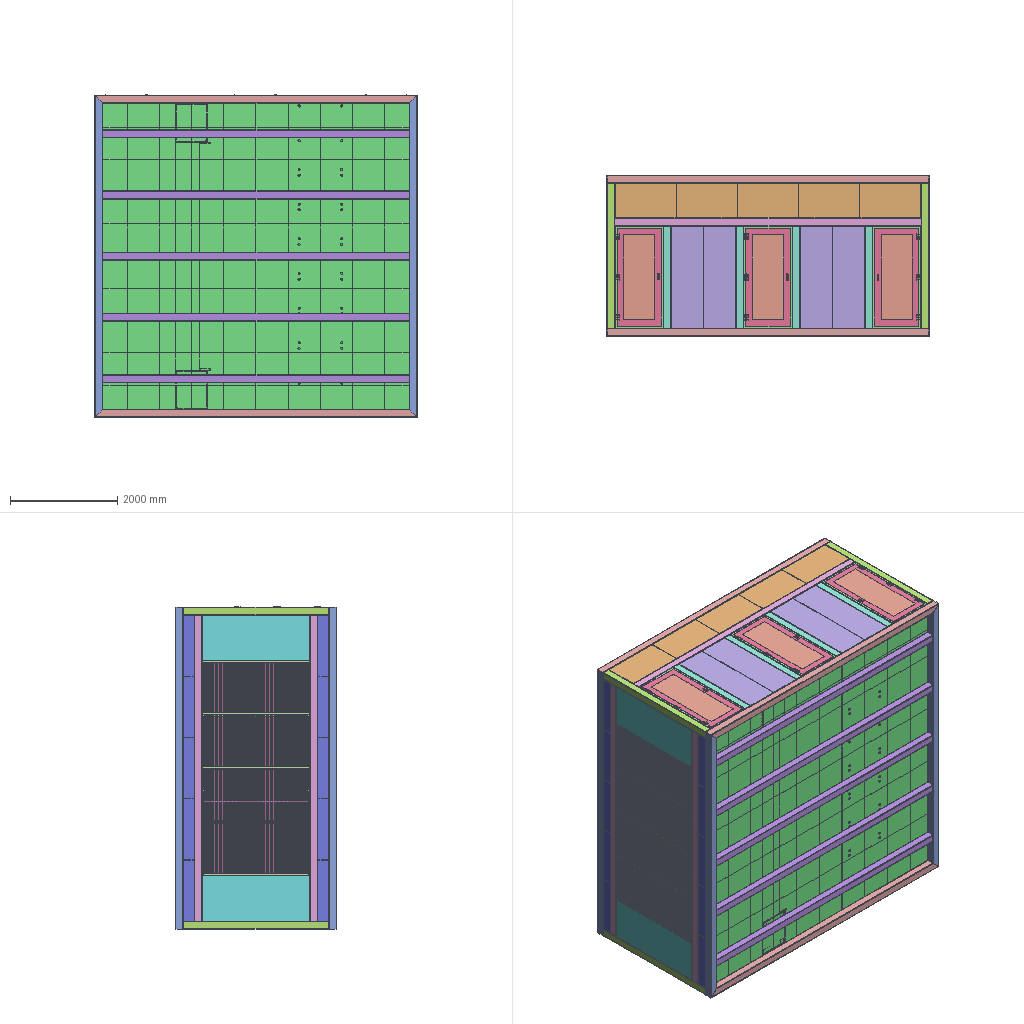Assembly | SolidWorks | 117 different items | 1806 placed | box 6000 x 3000 x 6007 mm
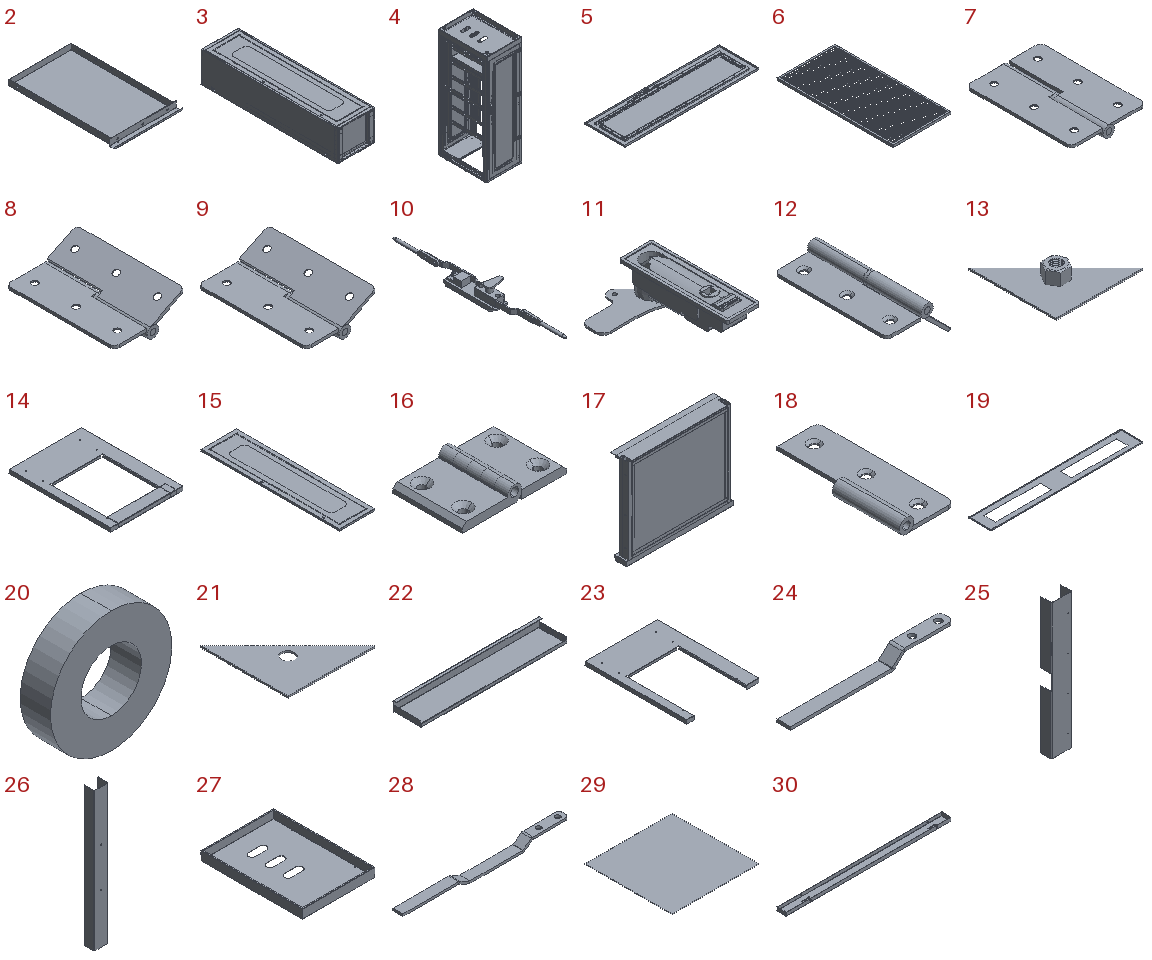Parts list (item | name | quantity | parent item | size | volume | features):
1 | 5.11-Top Cover | x1 | - | - | - | -
2 | (subassembly) | x9 | in 4 | 455 x 749 x 44.3 mm | 848864 mm3 | -
3 | (subassembly) | x2 | - | - | 30600871 mm3 | features ReferencePattern 9, MirrorCompFeat 5, LocalLPattern 2, AEMSimFeature 1
4 | (subassembly) | x9 | - | - | 20009952 mm3 | features ReferencePattern 2, LocalLPattern 1
5 | (subassembly) | x18 | in 4 | 1891 x 561 x 53 mm | 5274116 mm3 | -
6 | (subassembly) | x4 | - | 1000 x 2000 x 40 mm | 5519371 mm3 | features ReferencePattern 76, LocalLPattern 1
7 | (subassembly) | x1 | - | 80 x 113.6 x 12.2 mm | 35964 mm3 | -
8 | (subassembly) | x1 | - | 74.417 x 113.6 x 29.403 mm | 35964 mm3 | -
9 | (subassembly) | x1 | - | 74.417 x 113.6 x 29.403 mm | 35964 mm3 | -
10 | (subassembly) | x18 | in 5 | 52.826 x 480.757 x 53 mm | 142243 mm3 | -
11 | (subassembly) | x3 | - | 92 x 126.5 x 42.2 mm | 56869 mm3 | features AEMSimFeature 1
12 | (subassembly) | x7 | - | 66.654 x 113.6 x 38.247 mm | 35964 mm3 | features AEMSimFeature 1
13 | (subassembly) | x36 | in 4 | 100 x 100 x 17 mm | 13913 mm3 | -
14 | (subassembly) | x9 | in 4 | 645 x 900 x 35 mm | 1036306 mm3 | -
15 | (subassembly) | x2 | in 3 | 666 x 2594 x 35 mm | 4997012 mm3 | features MirrorCompFeat 6, ReferencePattern 4, AEMSimFeature 1
16 | (subassembly) | x54 | in 4 | 75.946 x 50 x 12.481 mm | 21969 mm3 | -
17 | (subassembly) | x14 | in 3 | 590 x 100 x 495 mm | 1096405 mm3 | features MirrorCompFeat 3, ReferencePattern 3, AEMSimFeature 1
18 | - | x7 | in 12 | 46.1 x 113.3 x 12.2 mm | 16282 mm3 | features BaseBody 1
19 | - | x1 | - | 5700 x 825 x 40 mm | 6847674 mm3 | features Cut 1, EdgeFlange 1, FlatPattern 1, SMBaseFlange 1, SheetMetal 1
20 | - | x7 | in 12 | 12 x 3 x 12 mm | 254.469 mm3 | features BaseBody 1
21 | - | x36 | in 13 | 100 x 100 x 2 mm | 9647 mm3 | features FlatPattern 1, SMBaseFlange 1, SheetMetal 1
22 | - | x9 | in 14 | 517 x 100 x 35 mm | 161621 mm3 | features EdgeFlange 4, FlatPattern 1, ICE 1, SMBaseFlange 1, SheetMetal 1
23 | - | x9 | in 14 | 645 x 900 x 35 mm | 874685 mm3 | features ICE 6, EdgeFlange 5, FlatPattern 1, SMBaseFlange 1, SheetMetal 1
24 | - | x18 | in 10 | 155.607 x 13 x 13.607 mm | 6013 mm3 | features EdgeFlange 2, Fillet 1, FlatPattern 1, ICE 1, SMBaseFlange 1, SheetMetal 1
25 | - | x2 | in 3 | 88 x 47.5 x 585 mm | 151349 mm3 | features ICE 2, Cut 1, FlatPattern 1, SMBaseFlange 1, SheetMetal 1
26 | - | x2 | in 3 | 63 x 45 x 621 mm | 137867 mm3 | features Cut 1, EdgeFlange 1, FlatPattern 1, SMBaseFlange 1, SheetMetal 1
27 | - | x9 | in 4 | 645 x 900 x 80 mm | 1637213 mm3 | features EdgeFlange 2, ICE 2, FlatPattern 1, SMBaseFlange 1, SheetMetal 1
28 | - | x18 | in 10 | 216.882 x 13 x 11.604 mm | 8395 mm3 | features EdgeFlange 4, Fillet 1, FlatPattern 1, ICE 1, SMBaseFlange 1, SheetMetal 1
29 | - | x100 | - | 600 x 600 x 2 mm | 720000 mm3 | features Extrusion 1
30 | - | x54 | in 4 | 850 x 50 x 18 mm | 137852 mm3 | features ICE 2, EdgeFlange 1, FlatPattern 1, SMBaseFlange 1, SheetMetal 1
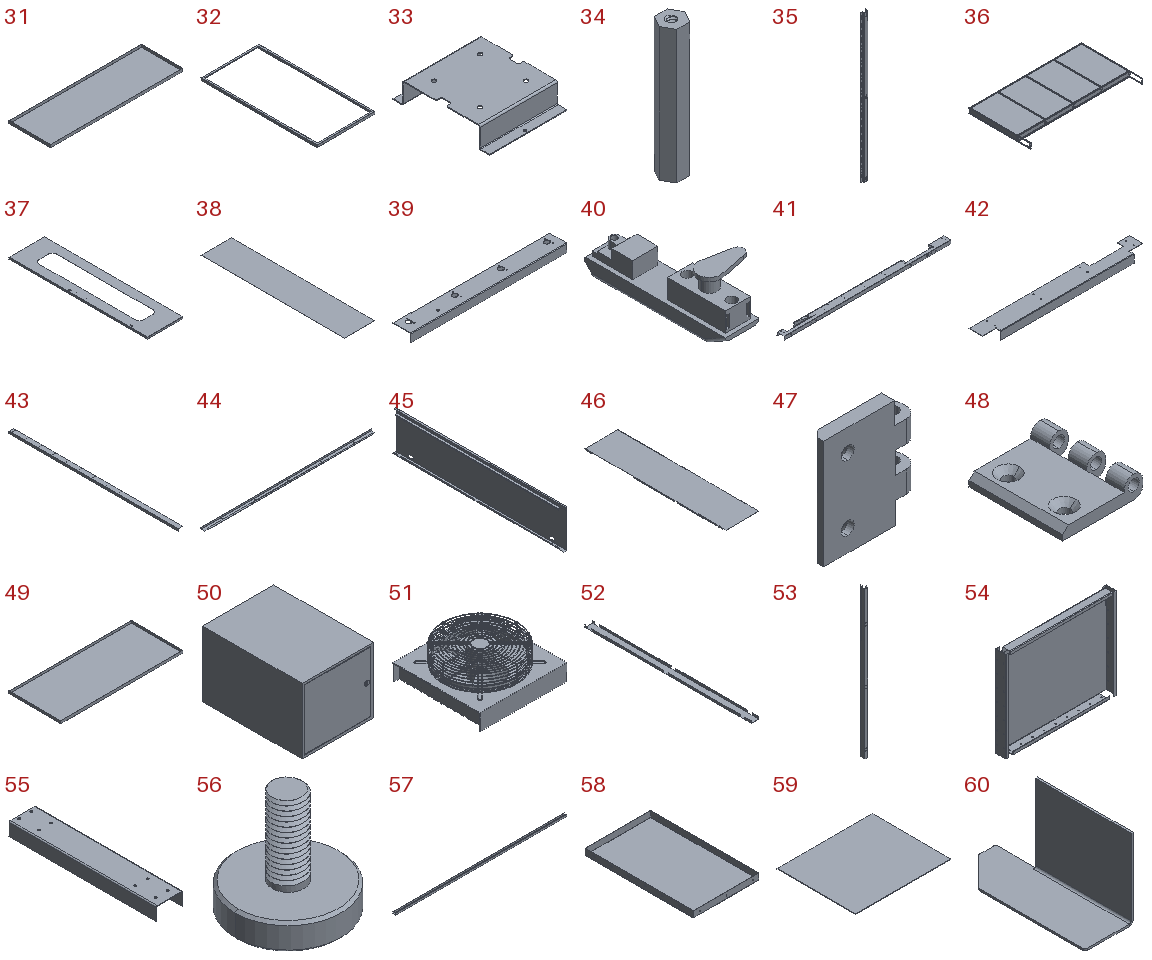31 | - | x4 | - | 1900 x 600 x 40 mm | 2650874 mm3 | features EdgeFlange 1, FlatPattern 1, SMBaseFlange 1, SheetMetal 1
32 | - | x4 | in 6 | 1000 x 2000 x 40 mm | 1030589 mm3 | features EdgeFlange 2, FlatPattern 1, ICE 1, SMBaseFlange 1, SheetMetal 1
33 | - | x2 | in 3 | 150 x 187 x 41 mm | 58020 mm3 | features EdgeFlange 2, Fillet 2, ICE 2, Cut 1, FlatPattern 1, SMBaseFlange 1, SheetMetal 1
34 | - | x54 | in 4 | 18.475 x 16 x 95 mm | 19634 mm3 | features Helix 2, ICE 2, SweepCut 2, Extrusion 1
35 | - | x36 | in 4 | 68 x 25 x 1590 mm | 315901 mm3 | features ICE 3, FlatPattern 1, SMBaseFlange 1, SheetMetal 1
36 | - | x1 | - | 4240 x 2313 x 200 mm | 1102421042 mm3 | features ICE 2, LPattern 2, WeldMemberFeat 1, WeldmentFeature 1
37 | - | x2 | in 15 | 666 x 2594 x 35 mm | 2126222 mm3 | features Cut 8, EdgeFlange 2, ICE 2, FlatPattern 1, SMBaseFlange 1, SheetMetal 1
38 | - | x2 | in 15 | 514 x 2442 x 1.2 mm | 1506226 mm3 | features FlatPattern 1, SMBaseFlange 1, SheetMetal 1
39 | - | x2 | in 15 | 610 x 70 x 32 mm | 112951 mm3 | features Cut 2, EdgeFlange 1, FlatPattern 1, ICE 1, SMBaseFlange 1, SheetMetal 1
40 | - | x18 | in 10 | 52.826 x 145 x 53 mm | 113904 mm3 | features ICE 19, CutThin 2, Fillet 2, Chamfer 1, Extrusion 1
41 | - | x2 | in 15 | 1598 x 70 x 32 mm | 211642 mm3 | features Cut 6, EdgeFlange 1, Fillet 1, FlatPattern 1, SMBaseFlange 1, SheetMetal 1
42 | - | x2 | in 15 | 625 x 70 x 32 mm | 64779 mm3 | features Cut 2, EdgeFlange 1, FlatPattern 1, ICE 1, SMBaseFlange 1, SheetMetal 1
43 | - | x4 | in 15 | 70 x 2448 x 32 mm | 293569 mm3 | features Cut 1, EdgeFlange 1, FlatPattern 1, ICE 1, SMBaseFlange 1, SheetMetal 1
44 | - | x36 | in 5 | 1760 x 53.5 x 18 mm | 208432 mm3 | features ICE 5, EdgeFlange 3, FlatPattern 1, SMBaseFlange 1, SheetMetal 1
45 | - | x2 | in 3 | 68.5 x 2698 x 600 mm | 3118659 mm3 | features EdgeFlange 6, ICE 3, Fillet 1, FlatPattern 1, SMBaseFlange 1, SheetMetal 1
46 | - | x2 | in 3 | 630 x 2698 x 20 mm | 2655544 mm3 | features Cut 2, EdgeFlange 1, FlatPattern 1, SMBaseFlange 1, SheetMetal 1
47 | - | x54 | in 16 | 43 x 12 x 50 mm | 10590 mm3 | features ICE 6, Chamfer 2, Fillet 1, FlatPattern 1, SMBaseFlange 1, SheetMetal 1
48 | - | x54 | in 16 | 43 x 50 x 12 mm | 11378 mm3 | features ICE 5, Chamfer 2, Fillet 2, FlatPattern 1, SMBaseFlange 1, SheetMetal 1
49 | - | x2 | - | 2000 x 850 x 40 mm | 3823030 mm3 | features EdgeFlange 1, FlatPattern 1, SMBaseFlange 1, SheetMetal 1
50 | - | x9 | - | 645 x 910 x 594.5 mm | 344886947 mm3 | features ICE 6, Extrusion 1
51 | - | x8 | - | 800 x 800 x 307.5 mm | 29684405 mm3 | features BaseBody 44, ICE 1
52 | - | x4 | in 3 | 80 x 1729 x 23 mm | 303401 mm3 | features ICE 2, FlatPattern 1, SMBaseFlange 1, SheetMetal 1
53 | - | x9 | in 4 | 54 x 73 x 1895 mm | 607316 mm3 | features ICE 2, FlatPattern 1, SMBaseFlange 1, SheetMetal 1
54 | - | x2 | in 3 | 726 x 68.5 x 598.5 mm | 957330 mm3 | features EdgeFlange 7, Cut 3, ICE 2, FlatPattern 1, SMBaseFlange 1, SheetMetal 1
55 | - | x4 | in 3 | 100 x 550 x 50 mm | 211963 mm3 | features EdgeFlange 1, FlatPattern 1, ICE 1, SMBaseFlange 1, SheetMetal 1
56 | - | x36 | in 4 | 40 x 40 x 40 mm | 15302 mm3 | features Chamfer 1, Extrusion 1, Helix 1, ICE 1, SweepCut 1
57 | - | x36 | in 5 | 1445 x 25 x 16 mm | 113630 mm3 | features EdgeFlange 1, FlatPattern 1, ICE 1, SMBaseFlange 1, SheetMetal 1
58 | - | x9 | in 2 | 425 x 700 x 40 mm | 758526 mm3 | features ICE 2, Extrusion 1, FlatPattern 1, FlattenBends 1, ProcessBends 1, Rip 1, SheetMetal 1, Shell 1
59 | - | x14 | in 17 | 531 x 440 x 3 mm | 700920 mm3 | features FlatPattern 1, SMBaseFlange 1, SheetMetal 1
60 | - | x14 | in 17 | 24 x 68 x 40 mm | 3346 mm3 | features EdgeFlange 1, FlatPattern 1, SMBaseFlange 1, SheetMetal 1
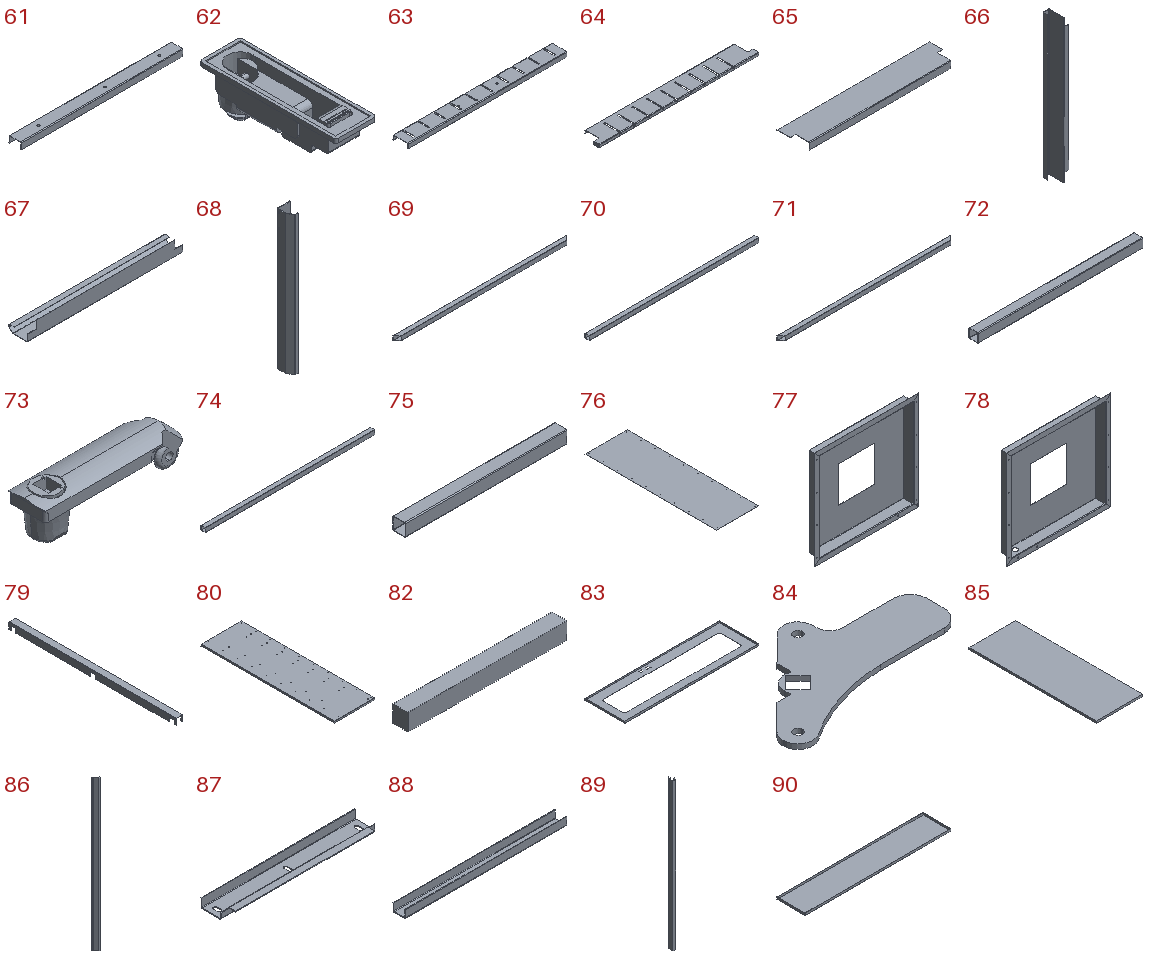61 | - | x14 | in 17 | 470 x 35 x 19 mm | 32665 mm3 | features EdgeFlange 1, FlatPattern 1, ICE 1, SMBaseFlange 1, SheetMetal 1
62 | - | x3 | in 11 | 35 x 117 x 42.2 mm | 38126 mm3 | features BaseBody 1
63 | - | x14 | in 17 | 526 x 50 x 15 mm | 37885 mm3 | features Cut 1, EdgeFlange 1, FlatPattern 1, Fold 1, ICE 1, SMBaseFlange 1, SheetMetal 1, UnFold 1
64 | - | x14 | in 17 | 567 x 70 x 10 mm | 44370 mm3 | features Cut 1, EdgeFlange 1, Fillet 1, FlatPattern 1, Fold 1, ICE 1, SMBaseFlange 1, SheetMetal 1, UnFold 1
65 | - | x14 | in 17 | 567 x 100 x 25 mm | 66763 mm3 | features Cut 1, EdgeFlange 1, FlatPattern 1, SMBaseFlange 1, SheetMetal 1
66 | - | x14 | in 17 | 34 x 51 x 470 mm | 44348 mm3 | features EdgeFlange 3, Fillet 1, FlatPattern 1, SMBaseFlange 1, SheetMetal 1
67 | - | x14 | in 17 | 590 x 70 x 55 mm | 85749 mm3 | features Cut 2, EdgeFlange 1, Fillet 1, FlatPattern 1, SMBaseFlange 1, SheetMetal 1
68 | - | x9 | in 2 | 42 x 49 x 455 mm | 90338 mm3 | features ICE 2, FlatPattern 1, SMBaseFlange 1, SheetMetal 1
69 | - | x4 | - | 6000 x 150 x 150 mm | 16588374 mm3 | features ICE 1, WeldMemberFeat 1, WeldmentFeature 1
70 | - | x10 | - | 5700 x 150 x 150 mm | 16163031 mm3 | features WeldMemberFeat 1, WeldmentFeature 1
71 | - | x4 | - | 6000 x 150 x 150 mm | 16588374 mm3 | features ICE 1, WeldMemberFeat 1, WeldmentFeature 1
72 | - | x4 | - | 2700 x 150 x 150 mm | 7656173 mm3 | features WeldMemberFeat 1, WeldmentFeature 1
73 | - | x3 | in 11 | 83.993 x 20.5 x 22.3 mm | 13621 mm3 | features BaseBody 1
74 | - | x3 | - | 5700 x 150 x 150 mm | 16163031 mm3 | features WeldMemberFeat 1, WeldmentFeature 1
75 | - | x4 | - | 1900 x 150 x 150 mm | 5387677 mm3 | features WeldMemberFeat 1, WeldmentFeature 1
76 | - | x2 | in 3 | 552 x 1731 x 1.2 mm | 1146313 mm3 | features FlatPattern 1, ICE 1, SMBaseFlange 1, SheetMetal 1
77 | - | x2 | in 3 | 552.6 x 55 x 523.6 mm | 424504 mm3 | features CornerFeat 4, EdgeFlange 3, ICE 2, Cut 1, Fillet 1, FlatPattern 1, SMBaseFlange 1, SheetMetal 1
78 | - | x2 | in 3 | 552.6 x 55 x 523.6 mm | 423620 mm3 | features EdgeFlange 3, ICE 3, CornerFeat 2, Cut 1, Fillet 1, FlatPattern 1, SMBaseFlange 1, SheetMetal 1
79 | - | x6 | in 3 | 70 x 1729 x 65.5 mm | 490504 mm3 | features Fillet 1, FlatPattern 1, ICE 1, SMBaseFlange 1, SheetMetal 1
80 | - | x2 | in 3 | 525 x 1733 x 21 mm | 1153064 mm3 | features Cut 2, EdgeFlange 1, FlatPattern 1, ICE 1, SMBaseFlange 1, SheetMetal 1
81 | - | x4 | - | - | - | features LPattern 1, Sweep 1, WeldMemberFeat 1, WeldmentFeature 1
82 | - | x1 | - | 4240 x 400 x 450 mm | 763200000 mm3 | features Extrusion 1
83 | - | x18 | in 5 | 1891 x 561 x 25 mm | 1274365 mm3 | features ICE 3, Extrusion 1, FlatPattern 1, FlattenBends 1, ProcessBends 1, Rip 1, SheetMetal 1, Shell 1
84 | - | x3 | in 11 | 92 x 54 x 2.3 mm | 5122 mm3 | features BaseBody 1
85 | - | x3 | - | 580 x 1580 x 25 mm | 22910000 mm3 | features Extrusion 1, ICE 1
86 | - | x308 | in 6 | 30 x 23 x 940 mm | 58296 mm3 | features FlatPattern 1, SMBaseFlange 1, SheetMetal 1
87 | - | x36 | in 5 | 305 x 53.5 x 18 mm | 35601 mm3 | features EdgeFlange 3, ICE 3, FlatPattern 1, SMBaseFlange 1, SheetMetal 1
88 | - | x36 | in 5 | 320 x 25 x 16 mm | 25103 mm3 | features EdgeFlange 1, FlatPattern 1, ICE 1, SMBaseFlange 1, SheetMetal 1
89 | - | x27 | in 4 | 54 x 73 x 1895 mm | 607655 mm3 | features FlatPattern 1, ICE 1, SMBaseFlange 1, SheetMetal 1
90 | - | x22 | - | 2700 x 518 x 40 mm | 3275069 mm3 | features EdgeFlange 1, FlatPattern 1, SMBaseFlange 1, SheetMetal 1
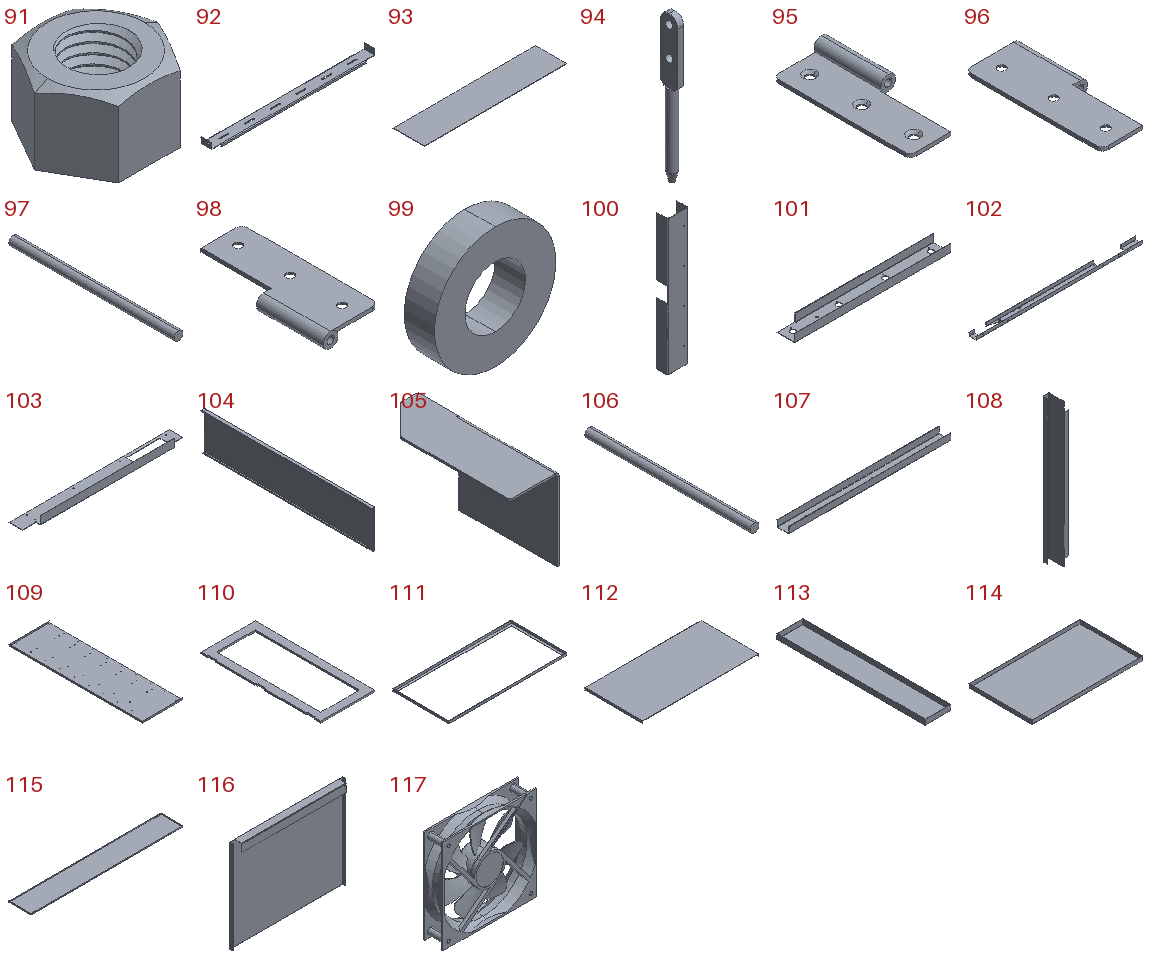91 | - | x36 | in 13 | 25.403 x 22 x 15 mm | 4267 mm3 | features Extrusion 1, Helix 1, ICE 1, RevCut 1, SweepCut 1
92 | - | x108 | in 4 | 700 x 50 x 33 mm | 87725 mm3 | features ICE 6, EdgeFlange 2, FlatPattern 1, SMBaseFlange 1, SheetMetal 1
93 | - | x18 | in 5 | 1685 x 367 x 5 mm | 3091975 mm3 | features FlatPattern 1, SMBaseFlange 1, SheetMetal 1
94 | - | x36 | in 10 | 8 x 15 x 125 mm | 6966 mm3 | features ICE 2, Chamfer 1, Extrusion 1, Fillet 1, RevCut 1
95 | - | x7 | in 12 | 46.1 x 113.3 x 12.2 mm | 16282 mm3 | features BaseBody 1
96 | - | x3 | in 7, 8, 9 | 46.1 x 113.3 x 12.2 mm | 16282 mm3 | features MirrorStock 1
97 | - | x3 | in 7, 8, 9 | 6 x 111.3 x 6 mm | 3147 mm3 | features MirrorStock 1
98 | - | x3 | in 7, 8, 9 | 46.1 x 113.3 x 12.2 mm | 16282 mm3 | features MirrorStock 1
99 | - | x3 | in 7, 8, 9 | 12 x 3 x 12 mm | 254.469 mm3 | features MirrorStock 1
100 | - | x2 | in 3 | 88 x 47.5 x 585 mm | 151349 mm3 | features MirrorStock 1
101 | - | x2 | in 15 | 610 x 70 x 32 mm | 112948 mm3 | features Cut 1, FlatPattern 1, MirrorStock 1, SMBaseFlange 1, SheetMetal 1, SolidToSheetMetal 1
102 | - | x2 | in 15 | 1598 x 70 x 32 mm | 211642 mm3 | features MirrorStock 1
103 | - | x2 | in 15 | 625 x 70 x 32 mm | 63464 mm3 | features ICE 2, FlatPattern 1, MirrorStock 1, SMBaseFlange 1, SheetMetal 1, SolidToSheetMetal 1
104 | - | x2 | in 3 | 68.5 x 2698 x 600 mm | 3118659 mm3 | features MirrorStock 1
105 | - | x14 | in 17 | 24 x 68 x 40 mm | 3346 mm3 | features MirrorStock 1
106 | - | x7 | in 12 | 6 x 111.3 x 6 mm | 3147 mm3 | features BaseBody 1
107 | - | x14 | in 17 | 470 x 35 x 19 mm | 32665 mm3 | features MirrorStock 1
108 | - | x14 | in 17 | 34 x 51 x 470 mm | 44348 mm3 | features MirrorStock 1
109 | - | x2 | in 3 | 525 x 1733 x 21 mm | 1153064 mm3 | features MirrorStock 1
110 | - | x3 | - | 820 x 1820 x 25 mm | 14268375 mm3 | features ICE 2, Extrusion 1
111 | - | x3 | - | 1900 x 900 x 40 mm | 850779 mm3 | features EdgeFlange 1, FlatPattern 1, ICE 1, SMBaseFlange 1, SheetMetal 1
112 | - | x1 | - | 4008 x 2000 x 80 mm | 16656000 mm3 | features ICE 2, Extrusion 1
113 | - | x10 | - | 200 x 1140 x 40 mm | 654012 mm3 | features EdgeFlange 1, FlatPattern 1, SMBaseFlange 1, SheetMetal 1
114 | - | x5 | - | 1140 x 650 x 40 mm | 1747070 mm3 | features EdgeFlange 1, FlatPattern 1, SMBaseFlange 1, SheetMetal 1
115 | - | x5 | - | 5700 x 825 x 40 mm | 10375674 mm3 | features EdgeFlange 1, FlatPattern 1, SMBaseFlange 1, SheetMetal 1
116 | - | x2 | in 3 | 726 x 50 x 598 mm | 777443 mm3 | features EdgeFlange 3, Cut 1, FlatPattern 1, ICE 1, SMBaseFlange 1, SheetMetal 1
117 | - | x10 | - | 420 x 87.5 x 420 mm | 2233634 mm3 | features BaseBody 2, CombineBodies 1, Scale 1
Mates (type | each side: item.copy, entity, surface, feature), first 313 of 386 lines:
In the top assembly
Coincident | 69.1 face plane Gb/6728-1986 Square Hollow Steel Section 150 X 150 X 5(1) | assembly plane
Coincident | 69.1 plane | assembly plane
Coincident | 69.1 face plane Gb/6728-1986 Square Hollow Steel Section 150 X 150 X 5(1) | 71.1 face plane Gb/6728-1986 Square Hollow Steel Section 150 X 150 X 5(1)
Coincident | 69.1 face plane Cut-Extrude 1 | 71.1 face plane Cut-Extrude 1
Coincident | 69.1 edge | 71.1 edge
Coincident | 71.1 plane | assembly plane
Coincident | 69.1 face plane Gb/6728-1986 Square Hollow Steel Section 150 X 150 X 5(1) | 72.1 face plane Gb/6728-1986 Square Hollow Steel Section 150 X 150 X 5(1) | 2 times
Coincident | 71.1 face plane Gb/6728-1986 Square Hollow Steel Section 150 X 150 X 5(1) | 72.1 face plane Gb/6728-1986 Square Hollow Steel Section 150 X 150 X 5(1)
Coincident | 69.2 face plane Gb/6728-1986 Square Hollow Steel Section 150 X 150 X 5(1) | 74.1 face plane Gb/6728-1986 Square Hollow Steel Section 150 X 150 X 5(1)
DistanceDim | 74.1 face plane Gb/6728-1986 Square Hollow Steel Section 150 X 150 X 5(1) | 69.2 face plane Gb/6728-1986 Square Hollow Steel Section 150 X 150 X 5(1)
Coincident | 72.1 face plane Gb/6728-1986 Square Hollow Steel Section 150 X 150 X 5(1) | 74.1 face plane Gb/6728-1986 Square Hollow Steel Section 150 X 150 X 5(1)
Coincident | 69.1 face plane Gb/6728-1986 Square Hollow Steel Section 150 X 150 X 5(1) | 75.1 face plane Gb/6728-1986 Square Hollow Steel Section 150 X 150 X 5(1) | 2 times
Coincident | 75.1 face plane Gb/6728-1986 Square Hollow Steel Section 150 X 150 X 5(1) | 75.2 face plane Gb/6728-1986 Square Hollow Steel Section 150 X 150 X 5(1)
Coincident | 69.1 face plane Gb/6728-1986 Square Hollow Steel Section 150 X 150 X 5(1) | 75.2 face plane Gb/6728-1986 Square Hollow Steel Section 150 X 150 X 5(1)
Coincident | 75.3 face plane Gb/6728-1986 Square Hollow Steel Section 150 X 150 X 5(1) | 75.4 face plane Gb/6728-1986 Square Hollow Steel Section 150 X 150 X 5(1) | 2 times
Coincident | 69.1 face plane Gb/6728-1986 Square Hollow Steel Section 150 X 150 X 5(1) | 75.3 face plane Gb/6728-1986 Square Hollow Steel Section 150 X 150 X 5(1)
Coincident | 75.2 face plane Gb/6728-1986 Square Hollow Steel Section 150 X 150 X 5(1) | 75.3 face plane Gb/6728-1986 Square Hollow Steel Section 150 X 150 X 5(1)
DistanceDim | 72.1 face plane Gb/6728-1986 Square Hollow Steel Section 150 X 150 X 5(1) | 75.2 face plane Gb/6728-1986 Square Hollow Steel Section 150 X 150 X 5(1)
DistanceDim | 72.2 face plane Gb/6728-1986 Square Hollow Steel Section 150 X 150 X 5(1) | 75.1 face plane Gb/6728-1986 Square Hollow Steel Section 150 X 150 X 5(1)
DistanceDim | 75.3 face plane Gb/6728-1986 Square Hollow Steel Section 150 X 150 X 5(1) | 75.4 face plane Gb/6728-1986 Square Hollow Steel Section 150 X 150 X 5(1)
Width | 75.3 face plane Gb/6728-1986 Square Hollow Steel Section 150 X 150 X 5(1) | 75.4 face plane Gb/6728-1986 Square Hollow Steel Section 150 X 150 X 5(1) | 75.2 face plane Gb/6728-1986 Square Hollow Steel Section 150 X 150 X 5(1) | 75.1 face plane Gb/6728-1986 Square Hollow Steel Section 150 X 150 X 5(1)
Coincident | 74.1 face plane Gb/6728-1986 Square Hollow Steel Section 150 X 150 X 5(1) | 114.1 face plane Base-Flange 1
Coincident | 74.1 face plane Gb/6728-1986 Square Hollow Steel Section 150 X 150 X 5(1) | 114.1 face plane Edge-Flange 1
Coincident | 72.1 face plane Gb/6728-1986 Square Hollow Steel Section 150 X 150 X 5(1) | 114.1 face plane Edge-Flange 1
Coincident | 69.1 face plane Gb/6728-1986 Square Hollow Steel Section 150 X 150 X 5(1) | 31.1 face plane Base-Flange 1
Coincident | 69.1 face plane Gb/6728-1986 Square Hollow Steel Section 150 X 150 X 5(1) | 31.1 face plane Edge-Flange 1
Coincident | 75.2 face plane Gb/6728-1986 Square Hollow Steel Section 150 X 150 X 5(1) | 31.1 face plane Edge-Flange 1
Coincident | 31.1 face plane Base-Flange 1 | 31.2 face plane Base-Flange 1
Coincident | 69.1 face plane Gb/6728-1986 Square Hollow Steel Section 150 X 150 X 5(1) | 31.2 face plane Edge-Flange 1
Coincident | 31.1 face plane Edge-Flange 1 | 31.2 face plane Edge-Flange 1
Coincident | 69.1 face plane Gb/6728-1986 Square Hollow Steel Section 150 X 150 X 5(1) | 111.1 face plane Base-Flange 1
Coincident | 69.1 face plane Gb/6728-1986 Square Hollow Steel Section 150 X 150 X 5(1) | 111.1 face plane Edge-Flange 1
Coincident | 72.1 face plane Gb/6728-1986 Square Hollow Steel Section 150 X 150 X 5(1) | 111.1 face plane Edge-Flange 1
Coincident | 69.1 face plane Gb/6728-1986 Square Hollow Steel Section 150 X 150 X 5(1) | 111.2 face plane Base-Flange 1
Coincident | 69.1 face plane Gb/6728-1986 Square Hollow Steel Section 150 X 150 X 5(1) | 111.2 face plane Edge-Flange 1
Coincident | 75.4 face plane Gb/6728-1986 Square Hollow Steel Section 150 X 150 X 5(1) | 111.2 face plane Edge-Flange 1
Coincident | 111.1 face plane Base-Flange 1 | 95.1 face plane SHHPSR845-3-SST_l(1)
DistanceDim | 12.1 plane | 111.1 face plane Edge-Flange 1
Symmetric | 69.1 face plane Gb/6728-1986 Square Hollow Steel Section 150 X 150 X 5(1) | 74.1 face plane Gb/6728-1986 Square Hollow Steel Section 150 X 150 X 5(1) | 12.1 plane
Parallel | 111.1 face plane Base-Flange 1 | 18.1 face plane SHHPSR845-3-SST_r(1)
Coincident | 111.1 face plane Cut-Extrude 1 | 110.1 face plane Boss-Extrude 1 | 2 times
Coincident | 111.1 face plane Base-Flange 1 | 110.1 face plane Boss-Extrude 1
Coincident | 110.1 face plane Boss-Extrude 1 | 85.1 face plane Boss-Extrude 1
Coincident | 110.1 face plane Cut-Extrude 1 | 85.1 face plane Cut-Extrude 1 | 2 times
Coincident | 71.1 face plane Gb/6728-1986 Square Hollow Steel Section 150 X 150 X 5(1) | 74.2 face plane Gb/6728-1986 Square Hollow Steel Section 150 X 150 X 5(1)
Coincident | 72.1 face plane Gb/6728-1986 Square Hollow Steel Section 150 X 150 X 5(1) | 74.2 face plane Gb/6728-1986 Square Hollow Steel Section 150 X 150 X 5(1)
DistanceDim | 74.2 face plane Gb/6728-1986 Square Hollow Steel Section 150 X 150 X 5(1) | 71.1 face plane Gb/6728-1986 Square Hollow Steel Section 150 X 150 X 5(1)
Coincident | 74.2 face plane Gb/6728-1986 Square Hollow Steel Section 150 X 150 X 5(1) | 74.3 face plane Gb/6728-1986 Square Hollow Steel Section 150 X 150 X 5(1)
Coincident | 72.1 face plane Gb/6728-1986 Square Hollow Steel Section 150 X 150 X 5(1) | 74.3 face plane Gb/6728-1986 Square Hollow Steel Section 150 X 150 X 5(1)
DistanceDim | 74.3 face plane Gb/6728-1986 Square Hollow Steel Section 150 X 150 X 5(1) | 71.2 face plane Gb/6728-1986 Square Hollow Steel Section 150 X 150 X 5(1)
Symmetric | 71.1 face plane Gb/6728-1986 Square Hollow Steel Section 150 X 150 X 5(1) | 74.2 face plane Gb/6728-1986 Square Hollow Steel Section 150 X 150 X 5(1) | 113.1 plane
Coincident | 74.2 face plane Gb/6728-1986 Square Hollow Steel Section 150 X 150 X 5(1) | 113.1 face plane Base-Flange 1
Coincident | 72.3 face plane Gb/6728-1986 Square Hollow Steel Section 150 X 150 X 5(1) | 113.1 face plane Edge-Flange 1
Coincident | 74.3 face plane Gb/6728-1986 Square Hollow Steel Section 150 X 150 X 5(1) | 113.2 face plane Base-Flange 1
Coincident | 72.3 face plane Gb/6728-1986 Square Hollow Steel Section 150 X 150 X 5(1) | 113.2 face plane Edge-Flange 1
Coincident | 71.2 face plane Gb/6728-1986 Square Hollow Steel Section 150 X 150 X 5(1) | 113.2 face plane Edge-Flange 1
Coincident | 74.2 face plane Gb/6728-1986 Square Hollow Steel Section 150 X 150 X 5(1) | 32.1 face plane Base-Flange 1
Coincident | 74.2 face plane Gb/6728-1986 Square Hollow Steel Section 150 X 150 X 5(1) | 32.1 face plane Edge-Flange 1
Width | 32.1 face plane Edge-Flange 1 | 32.2 face plane Edge-Flange 1 | 72.3 face plane Gb/6728-1986 Square Hollow Steel Section 150 X 150 X 5(1) | 72.1 face plane Gb/6728-1986 Square Hollow Steel Section 150 X 150 X 5(1)
Coincident | 74.2 face plane Gb/6728-1986 Square Hollow Steel Section 150 X 150 X 5(1) | 49.1 face plane Base-Flange 1
Coincident | 74.2 face plane Gb/6728-1986 Square Hollow Steel Section 150 X 150 X 5(1) | 49.1 face plane Edge-Flange 1
Coincident | 72.3 face plane Gb/6728-1986 Square Hollow Steel Section 150 X 150 X 5(1) | 49.1 face plane Edge-Flange 1
Coincident | 74.2 face plane Gb/6728-1986 Square Hollow Steel Section 150 X 150 X 5(1) | 49.2 face plane Edge-Flange 1
Coincident | 74.2 face plane Gb/6728-1986 Square Hollow Steel Section 150 X 150 X 5(1) | 49.2 face plane Base-Flange 1
Coincident | 72.1 face plane Gb/6728-1986 Square Hollow Steel Section 150 X 150 X 5(1) | 49.2 face plane Edge-Flange 1
Coincident | 69.3 face plane Gb/6728-1986 Square Hollow Steel Section 150 X 150 X 5(1) | 90.1 face plane Base-Flange 1 | 2 times
Coincident | 69.3 face plane Gb/6728-1986 Square Hollow Steel Section 150 X 150 X 5(1) | 90.1 face plane Edge-Flange 1
Width | 72.4 face plane Gb/6728-1986 Square Hollow Steel Section 150 X 150 X 5(1) | 72.3 face plane Gb/6728-1986 Square Hollow Steel Section 150 X 150 X 5(1) | 90.1 face plane Edge-Flange 1 | 90.2 face plane Edge-Flange 1
Coincident | 71.3 face plane Gb/6728-1986 Square Hollow Steel Section 150 X 150 X 5(1) | 90.3 face plane Base-Flange 1 | 2 times
Coincident | 71.3 face plane Gb/6728-1986 Square Hollow Steel Section 150 X 150 X 5(1) | 90.3 face plane Edge-Flange 1
Width | 72.2 face plane Gb/6728-1986 Square Hollow Steel Section 150 X 150 X 5(1) | 72.4 face plane Gb/6728-1986 Square Hollow Steel Section 150 X 150 X 5(1) | 90.3 face plane Edge-Flange 1 | 90.4 face plane Edge-Flange 1
Coincident | 69.3 face plane Gb/6728-1986 Square Hollow Steel Section 150 X 150 X 5(1) | 70.1 face plane Gb/6728-1986 Square Hollow Steel Section 150 X 150 X 5(1)
Coincident | 71.1 face plane Gb/6728-1986 Square Hollow Steel Section 150 X 150 X 5(1) | 70.1 face plane Gb/6728-1986 Square Hollow Steel Section 150 X 150 X 5(1)
Parallel | 90.1 face plane Base-Flange 1 | 29.1 face plane Boss-Extrude 1
Parallel | 90.5 face plane Base-Flange 1 | 29.1 face plane Boss-Extrude 1
Coincident | 70.1 face plane Gb/6728-1986 Square Hollow Steel Section 150 X 150 X 5(1) | 29.1 face plane Boss-Extrude 1
Width | 29.2 face plane Boss-Extrude 1 | 29.1 face plane Boss-Extrude 1 | 71.3 face plane Gb/6728-1986 Square Hollow Steel Section 150 X 150 X 5(1) | 71.1 face plane Gb/6728-1986 Square Hollow Steel Section 150 X 150 X 5(1)
Width | 29.3 face plane Boss-Extrude 1 | 29.1 face plane Boss-Extrude 1 | 69.3 face plane Gb/6728-1986 Square Hollow Steel Section 150 X 150 X 5(1) | 69.1 face plane Gb/6728-1986 Square Hollow Steel Section 150 X 150 X 5(1)
Width | 70.1 face plane Gb/6728-1986 Square Hollow Steel Section 150 X 150 X 5(1) | 70.2 face plane Gb/6728-1986 Square Hollow Steel Section 150 X 150 X 5(1) | 69.3 face plane Gb/6728-1986 Square Hollow Steel Section 150 X 150 X 5(1) | 69.1 face plane Gb/6728-1986 Square Hollow Steel Section 150 X 150 X 5(1)
Coincident | 69.2 face plane Gb/6728-1986 Square Hollow Steel Section 150 X 150 X 5(1) | 70.3 face plane Gb/6728-1986 Square Hollow Steel Section 150 X 150 X 5(1) | 2 times
Coincident | 70.3 plane | assembly plane
Coincident | 70.4 face plane Gb/6728-1986 Square Hollow Steel Section 150 X 150 X 5(1) | 70.5 face plane Gb/6728-1986 Square Hollow Steel Section 150 X 150 X 5(1) | 2 times
Coincident | 69.2 face plane Gb/6728-1986 Square Hollow Steel Section 150 X 150 X 5(1) | 70.4 face plane Gb/6728-1986 Square Hollow Steel Section 150 X 150 X 5(1)
Coincident | 71.2 face plane Gb/6728-1986 Square Hollow Steel Section 150 X 150 X 5(1) | 115.1 face plane Base-Flange 1
Coincident | 69.2 face plane Gb/6728-1986 Square Hollow Steel Section 150 X 150 X 5(1) | 115.1 face plane Edge-Flange 1
Coincident | 71.2 face plane Gb/6728-1986 Square Hollow Steel Section 150 X 150 X 5(1) | 115.1 face plane Edge-Flange 1
DistanceDim | 71.2 face plane Gb/6728-1986 Square Hollow Steel Section 150 X 150 X 5(1) | 70.4 face plane Gb/6728-1986 Square Hollow Steel Section 150 X 150 X 5(1)
Coincident | 70.4 face plane Gb/6728-1986 Square Hollow Steel Section 150 X 150 X 5(1) | 69.2 face plane Gb/6728-1986 Square Hollow Steel Section 150 X 150 X 5(1)
DistanceDim | 70.5 face plane Gb/6728-1986 Square Hollow Steel Section 150 X 150 X 5(1) | 70.4 face plane Gb/6728-1986 Square Hollow Steel Section 150 X 150 X 5(1)
Coincident | 71.4 face plane Gb/6728-1986 Square Hollow Steel Section 150 X 150 X 5(1) | 117.1 face plane Import 2
Parallel | 71.4 face plane Gb/6728-1986 Square Hollow Steel Section 150 X 150 X 5(1) | 117.1 face plane Import 2
Width | 117.2 face plane Import 2 | 117.2 face plane Import 2 | 70.6 face plane Gb/6728-1986 Square Hollow Steel Section 150 X 150 X 5(1) | 71.4 face plane Gb/6728-1986 Square Hollow Steel Section 150 X 150 X 5(1)
Coincident | 71.4 face plane Gb/6728-1986 Square Hollow Steel Section 150 X 150 X 5(1) | 19.1 face plane Base-Flange 1
Coincident | 69.2 face plane Gb/6728-1986 Square Hollow Steel Section 150 X 150 X 5(1) | 19.1 face plane Edge-Flange 1
Coincident | 70.6 face plane Gb/6728-1986 Square Hollow Steel Section 150 X 150 X 5(1) | 19.1 face plane Edge-Flange 1
Coincident | 51.1 face plane Import 38 | 51.2 face plane Import 38 | 2 times
Parallel | 115.2 face plane Base-Flange 1 | 51.1 face plane Import 38
Parallel | 114.2 face plane Base-Flange 1 | 51.1 face plane Import 38
Width | 51.1 face plane Import 38 | 51.3 face plane Import 38 | 69.4 face plane Gb/6728-1986 Square Hollow Steel Section 150 X 150 X 5(1) | 69.2 face plane Gb/6728-1986 Square Hollow Steel Section 150 X 150 X 5(1)
Coincident | 29.4 face plane Boss-Extrude 1 | 82.1 face plane Boss-Extrude 1
DistanceDim | 82.1 face plane Boss-Extrude 1 | 72.1 face plane Gb/6728-1986 Square Hollow Steel Section 150 X 150 X 5(1)
Coincident | 29.5 face plane Boss-Extrude 1 | 54.1 face plane Edge-Flange 8
Coincident | 82.1 face plane Boss-Extrude 1 | 45.1 face plane Edge-Flange 1
Coincident | 82.1 face plane Boss-Extrude 1 | 45.1 face plane Base-Flange 1
Coincident | 110.1 face plane Boss-Extrude 1 | 62.1 face plane E-PAT-117-D-S_b(1)
Coincident | 62.1 face plane E-PAT-117-D-S_b(1) | 62.2 face plane E-PAT-117-D-S_b(1)
Coincident | 62.2 face plane E-PAT-117-D-S_b(1) | 62.3 face plane E-PAT-117-D-S_b(1)
Coincident | 29.6 face plane Boss-Extrude 1 | 56.1 face plane Boss-Extrude 1
Parallel | 49.1 face plane Base-Flange 1 | 83.1 face plane Boss-Extrude 1
DistanceDim | 75.1 face plane Gb/6728-1986 Square Hollow Steel Section 150 X 150 X 5(1) | 89.1 face plane Base-Flange 1
Coincident | 74.1 face plane Gb/6728-1986 Square Hollow Steel Section 150 X 150 X 5(1) | 23.1 face plane Edge-Flange 1
Coincident | 51.2 face plane Import 38 | 82.1 face plane Boss-Extrude 1
Coincident | 49.2 face plane Base-Flange 1 | 112.1 face plane Boss-Extrude 2
Coincident | 49.2 face plane Edge-Flange 1 | 112.1 face plane Boss-Extrude 2
DistanceDim | 112.1 face plane Boss-Extrude 1 | 74.3 face plane Gb/6728-1986 Square Hollow Steel Section 150 X 150 X 5(1)
Coincident | 74.1 face plane Gb/6728-1986 Square Hollow Steel Section 150 X 150 X 5(1) | 104.1 face plane Right Side Mirror
Coincident | 36.1 plane | assembly plane
Coincident | 29.7 face plane Boss-Extrude 1 | 36.1 face plane LPattern 1
DistanceDim | 36.1 face plane Gb/6728-1986 Square Hollow Steel Section 025 X 25 X 1.75(1) | 45.2 face plane Edge-Flange 1
Coincident | 45.2 face plane Base-Flange 1 | 81.1 face plane Gb/6728-1986 Square Hollow Steel Section 050 X 50 X 3(1)
Coincident | 82.1 face plane Boss-Extrude 1 | 81.1 face plane Gb/6728-1986 Square Hollow Steel Section 050 X 50 X 3(1)
DistanceDim | 81.1 face plane Gb/6728-1986 Square Hollow Steel Section 050 X 50 X 3(1) | 82.1 face plane Boss-Extrude 1
In subassembly 12
Concentric | 106.1 face cylinder SHHPSR845-3-SST_p(1) | 18.2 face cylinder SHHPSR845-3-SST_r(1)
Coincident | 20.1 face plane WASHER12-6-3(1) | 18.2 face plane SHHPSR845-3-SST_r(1)
In subassembly 4
Coincident | 27.1 face plane Edge-Flange 3 | 21.1 face plane Base-Flange 1 | 3 times
Coincident | 27.1 face plane Edge-Flange 3 | 21.2 face plane Base-Flange 1 | 3 times
Coincident | 27.1 face plane Edge-Flange 3 | 21.3 face plane Base-Flange 1 | 3 times
Coincident | 27.1 face plane Edge-Flange 3 | 21.4 face plane Base-Flange 1 | 3 times
Coincident | 27.1 face plane Edge-Flange 1 | 89.2 face plane Base-Flange 1 | 2 times
Coincident | 27.1 face plane Base-Flange 1 | 89.2 face plane Base-Flange 1
Coincident | 27.1 face plane Edge-Flange 1 | 89.3 face plane Base-Flange 1 | 2 times
Coincident | 27.1 face plane Base-Flange 1 | 89.3 face plane Base-Flange 1
Coincident | 27.1 face plane Edge-Flange 1 | 89.4 face plane Base-Flange 1 | 2 times
Coincident | 27.1 face plane Base-Flange 1 | 89.4 face plane Base-Flange 1
Coincident | 89.3 face plane Base-Flange 1 | 23.2 face plane Edge-Flange 1 | 2 times
Coincident | 89.3 face plane Base-Flange 1 | 23.2 face plane Base-Flange 1
Coincident | 27.1 face plane Base-Flange 1 | 30.1 face plane Edge-Flange 1
Coincident | 89.3 face plane Base-Flange 1 | 30.1 face plane Edge-Flange 1 | 2 times
Coincident | 27.1 face plane Base-Flange 1 | 30.2 face plane Edge-Flange 1
Coincident | 89.4 face plane Base-Flange 1 | 30.2 face plane Base-Flange 1
Coincident | 89.4 face plane Base-Flange 1 | 30.2 face plane Edge-Flange 1
Coincident | 89.4 face plane Base-Flange 1 | 30.3 face plane Base-Flange 1
Coincident | 23.2 face plane Base-Flange 1 | 30.3 face plane Edge-Flange 1
Coincident | 89.4 face plane Base-Flange 1 | 30.3 face plane Edge-Flange 1
Coincident | 89.3 face plane Base-Flange 1 | 30.4 face plane Base-Flange 1
Coincident | 23.2 face plane Base-Flange 1 | 30.4 face plane Edge-Flange 1
Coincident | 89.3 face plane Base-Flange 1 | 30.4 face plane Edge-Flange 1
Coincident | 89.4 face plane Base-Flange 1 | 30.5 face plane Edge-Flange 1 | 2 times
Coincident | 89.3 face plane Base-Flange 1 | 30.6 face plane Base-Flange 1
Coincident | 89.3 face plane Base-Flange 1 | 30.6 face plane Edge-Flange 1
Coincident | 30.1 face plane Base-Flange 1 | 35.1 face plane Base-Flange 1
DistanceDim | 35.1 face plane Base-Flange 1 | 27.1 face plane Edge-Flange 1
Coincident | 30.2 face plane Base-Flange 1 | 35.2 face plane Base-Flange 1
DistanceDim | 35.2 face plane Base-Flange 1 | 27.1 face plane Edge-Flange 1
DistanceDim | 27.1 face plane Base-Flange 1 | 35.1 face plane Base-Flange 1
DistanceDim | 27.1 face plane Base-Flange 1 | 35.2 face plane Base-Flange 1
Coincident | 30.2 face plane Base-Flange 1 | 35.3 face plane Base-Flange 1
DistanceDim | 35.3 face plane Base-Flange 1 | 27.1 face plane Base-Flange 1
Coincident | 30.1 face plane Base-Flange 1 | 35.4 face plane Base-Flange 1
DistanceDim | 27.1 face plane Base-Flange 1 | 35.4 face plane Base-Flange 1
DistanceDim | 35.3 face plane Base-Flange 1 | 89.4 face plane Base-Flange 1
DistanceDim | 35.4 face plane Base-Flange 1 | 89.3 face plane Base-Flange 1
DistanceDim | 27.1 face plane Base-Flange 1 | 30.6 face plane Edge-Flange 1
DistanceDim | 30.5 face plane Edge-Flange 1 | 27.1 face plane Base-Flange 1
Coincident | 35.2 face plane Base-Flange 1 | 92.1 face plane Edge-Flange 3
DistanceDim | 92.1 face plane Edge-Flange 3 | 35.2 face plane Base-Flange 1
Coincident | 35.1 face plane Base-Flange 1 | 92.2 face plane Edge-Flange 3
DistanceDim | 35.1 face plane Base-Flange 1 | 92.2 face plane Edge-Flange 3
DistanceDim | 27.1 face plane Base-Flange 1 | 92.2 face plane Edge-Flange 2
DistanceDim | 27.1 face plane Base-Flange 1 | 92.1 face plane Edge-Flange 2
Coincident | 35.4 face plane Base-Flange 1 | 92.3 face plane Edge-Flange 3
DistanceDim | 92.3 face plane Edge-Flange 3 | 35.4 face plane Base-Flange 1
DistanceDim | 92.2 face plane Edge-Flange 2 | 92.3 face plane Edge-Flange 2
Coincident | 35.2 face plane Base-Flange 1 | 92.4 face plane Edge-Flange 3
DistanceDim | 92.4 face plane Edge-Flange 3 | 35.2 face plane Base-Flange 1
DistanceDim | 92.1 face plane Edge-Flange 2 | 92.4 face plane Edge-Flange 2
Coincident | 35.2 face plane Base-Flange 1 | 92.5 face plane Edge-Flange 3
DistanceDim | 92.5 face plane Edge-Flange 3 | 35.2 face plane Base-Flange 1
DistanceDim | 92.4 face plane Edge-Flange 2 | 92.5 face plane Edge-Flange 2
Coincident | 35.1 face plane Base-Flange 1 | 92.6 face plane Edge-Flange 3
DistanceDim | 92.3 face plane Edge-Flange 2 | 92.6 face plane Edge-Flange 2
DistanceDim | 92.6 face plane Edge-Flange 3 | 35.1 face plane Base-Flange 1
Coincident | 35.3 face plane Base-Flange 1 | 92.7 face plane Edge-Flange 3
DistanceDim | 92.7 face plane Edge-Flange 3 | 35.3 face plane Base-Flange 1
DistanceDim | 92.5 face plane Edge-Flange 2 | 92.7 face plane Edge-Flange 2
Coincident | 35.4 face plane Base-Flange 1 | 92.8 face plane Edge-Flange 3
DistanceDim | 92.8 face plane Edge-Flange 3 | 35.4 face plane Base-Flange 1
DistanceDim | 92.6 face plane Edge-Flange 2 | 92.8 face plane Edge-Flange 2
Coincident | 35.4 face plane Base-Flange 1 | 92.9 face plane Edge-Flange 3
DistanceDim | 35.4 face plane Base-Flange 1 | 92.9 face plane Edge-Flange 3
DistanceDim | 92.8 face plane Edge-Flange 2 | 92.9 face plane Edge-Flange 2
DistanceDim | 92.10 face plane Edge-Flange 3 | 35.3 face plane Base-Flange 1
Coincident | 35.3 face plane Base-Flange 1 | 92.10 face plane Edge-Flange 3
DistanceDim | 92.7 face plane Edge-Flange 2 | 92.10 face plane Edge-Flange 2
Coincident | 35.4 face plane Base-Flange 1 | 92.11 face plane Edge-Flange 3
DistanceDim | 92.11 face plane Edge-Flange 3 | 35.4 face plane Base-Flange 1
DistanceDim | 92.9 face plane Edge-Flange 2 | 92.11 face plane Edge-Flange 2
Coincident | 35.3 face plane Base-Flange 1 | 92.12 face plane Edge-Flange 3
DistanceDim | 92.12 face plane Edge-Flange 3 | 35.3 face plane Base-Flange 1
DistanceDim | 92.10 face plane Edge-Flange 2 | 92.12 face plane Edge-Flange 2
Concentric | 23.2 face cylinder Cut-Extrude 5 | 34.1 face cylinder Cut-Extrude 1
Coincident | 23.2 face plane Base-Flange 1 | 34.1 face plane Boss-Extrude 1
Concentric | 23.2 face cylinder Cut-Extrude 5 | 34.2 face cylinder Cut-Extrude 1
Coincident | 23.2 face plane Base-Flange 1 | 34.2 face plane Boss-Extrude 1
Concentric | 23.2 face cylinder Cut-Extrude 5 | 34.3 face cylinder Cut-Extrude 1
Coincident | 23.2 face plane Base-Flange 1 | 34.3 face plane Boss-Extrude 1
Concentric | 23.2 face cylinder Cut-Extrude 5 | 34.4 face cylinder Cut-Extrude 1
Coincident | 23.2 face plane Base-Flange 1 | 34.4 face plane Boss-Extrude 1
Concentric | 23.2 face cylinder Cut-Extrude 5 | 34.5 face cylinder Cut-Extrude 1
Coincident | 23.2 face plane Base-Flange 1 | 34.5 face plane Boss-Extrude 1
Concentric | 23.2 face cylinder Cut-Extrude 5 | 34.6 face cylinder Cut-Extrude 1
Coincident | 23.2 face plane Base-Flange 1 | 34.6 face plane Boss-Extrude 1
Concentric | 91.1 face cylinder Cut-Extrude 1 | 56.2 face cylinder Boss-Extrude 3
DistanceDim | 21.4 face plane Base-Flange 1 | 56.2 face plane Boss-Extrude 1
Concentric | 91.2 face cylinder Cut-Extrude 1 | 56.3 face cylinder Boss-Extrude 3
DistanceDim | 21.3 face plane Base-Flange 1 | 56.3 face plane Boss-Extrude 1
Concentric | 91.3 face cylinder Cut-Extrude 1 | 56.4 face cylinder Boss-Extrude 3 | 2 times
DistanceDim | 21.1 face plane Base-Flange 1 | 56.4 face plane Boss-Extrude 1
Concentric | 91.4 face cylinder Cut-Extrude 1 | 56.5 face cylinder Boss-Extrude 3
DistanceDim | 21.2 face plane Base-Flange 1 | 56.5 face plane Boss-Extrude 1
Coincident | 23.2 face plane Edge-Flange 1 | 53.1 face plane Base-Flange 1 | 2 times
Coincident | 23.2 face plane Base-Flange 1 | 53.1 face plane Base-Flange 1
Tangent | 89.4 face cylinder Base Bend 1 | 30.5 face plane Base-Flange 1
Concentric | 53.1 face cylinder Cut-Extrude 2 | 47.1 face cylinder Extrude 3 | 2 times
Coincident | 53.1 face plane Base-Flange 1 | 47.1 face plane Base-Flange 1
Concentric | 53.1 face cylinder Cut-Extrude 2 | 47.2 face cylinder Extrude 3 | 2 times
Coincident | 53.1 face plane Base-Flange 1 | 47.2 face plane Base-Flange 1
Concentric | 53.1 face cylinder Cut-Extrude 2 | 47.3 face cylinder Extrude 3 | 2 times
Coincident | 53.1 face plane Base-Flange 1 | 47.3 face plane Base-Flange 1
DistanceDim | 83.2 face plane Boss-Extrude 1 | 22.1 face plane Base-Flange 1
DistanceDim | 83.2 face plane Boss-Extrude 1 | 53.1 face plane Base-Flange 1
Coincident | 53.1 face plane Base-Flange 1 | 83.2 face plane Boss-Extrude 1
DistanceDim | 58.1 face plane Boss-Extrude 1 | 92.4 face plane Base-Flange 1
DistanceDim | 58.1 face plane Boss-Extrude 1 | 92.4 face plane Edge-Flange 2
Coincident | 83.2 face plane Boss-Extrude 1 | 83.3 face plane Boss-Extrude 1 | 2 times
Coincident | 89.4 face plane Base-Flange 1 | 83.3 face plane Boss-Extrude 1
Concentric | 83.3 face cylinder Cut-Extrude 1 | 48.1 face cylinder Extrude 4 | 2 times
In subassembly 13
Concentric | 21.5 face cylinder Base-Flange 1 | 91.5 face cylinder Cut-Extrude 1
Coincident | 21.5 face plane Base-Flange 1 | 91.5 face plane Boss-Extrude 1
In subassembly 14
Coincident | 23.3 face plane Base-Flange 1 | 22.2 face plane Base-Flange 1
Coincident | 23.3 face plane Edge-Flange 1 | 22.2 face plane Edge-Flange 1
Coincident | 23.3 face plane Edge-Flange 3 | 22.2 face plane Edge-Flange 4
In subassembly 16
Concentric | 48.2 face cylinder Extrude 3 | 47.4 face cylinder Extrude 2
Coincident | 48.2 face plane Extrude 6 | 47.4 face plane Extrude 10
In subassembly 5
Coincident | 83.4 face plane Shell 1 | 57.1 face plane Edge-Flange 1
DistanceDim | 57.1 face plane Edge-Flange 1 | 83.4 face plane Cut-Extrude 4
DistanceDim | 83.4 face plane Cut-Extrude 4 | 57.1 face plane Edge-Flange 1
Coincident | 83.4 face plane Shell 1 | 57.2 face plane Edge-Flange 1
DistanceDim | 57.2 face plane Edge-Flange 1 | 83.4 face plane Cut-Extrude 4 | 2 times
Coincident | 83.4 face plane Shell 1 | 88.1 face plane Edge-Flange 1
Coincident | 57.2 face plane Edge-Flange 1 | 88.1 face plane Edge-Flange 1
Coincident | 83.4 face plane Shell 1 | 88.2 face plane Edge-Flange 1
Coincident | 57.1 face plane Edge-Flange 1 | 88.2 face plane Edge-Flange 1 | 2 times
Coincident | 83.4 face plane Shell 1 | 87.1 face plane Edge-Flange 1
DistanceDim | 87.1 face plane Edge-Flange 1 | 88.1 face plane Edge-Flange 1
Coincident | 83.4 face plane Shell 1 | 87.2 face plane Edge-Flange 1
DistanceDim | 88.2 face plane Edge-Flange 1 | 87.2 face plane Edge-Flange 2
Coincident | 83.4 face plane Shell 1 | 44.1 face plane Edge-Flange 1
DistanceDim | 57.2 face plane Edge-Flange 1 | 44.1 face plane Edge-Flange 1
Coincident | 83.4 face plane Shell 1 | 44.2 face plane Edge-Flange 1
DistanceDim | 57.1 face plane Edge-Flange 1 | 44.2 face plane Edge-Flange 1
Coincident | 87.2 face plane Edge-Flange 1 | 44.2 face plane Base-Flange 1
Coincident | 83.4 face plane Shell 1 | 93.1 face plane Base-Flange 1
DistanceDim | 93.1 face plane Base-Flange 1 | 57.1 face plane Edge-Flange 1
Coincident | 83.4 face plane Boss-Extrude 1 | 40.1 face plane Boss-Extrude 1
Coincident | 83.4 face plane Cut-Extrude 5 | 40.1 face plane Boss-Extrude 2
Coincident | 83.4 face plane Cut-Extrude 5 | 40.1 face plane Boss-Extrude 3
Coincident | 44.1 face plane Base-Flange 1 | 44.2 face plane Edge-Flange 1
In subassembly 10
Coincident | 40.2 face plane Cut-Extrude 19 | 24.1 face plane Base-Flange 1 | 2 times
Coincident | 40.2 face plane Cut-Extrude 19 | 28.1 face plane Base-Flange 1 | 2 times
Concentric | 24.1 face cylinder Cut-Extrude 1 | 94.1 face cylinder Cut-Extrude 4 | 2 times
Coincident | 24.1 face plane Edge-Flange 2 | 94.1 face plane Boss-Extrude 2
Concentric | 28.1 face cylinder Cut-Extrude 1 | 94.2 face cylinder Cut-Extrude 4 | 2 times
Coincident | 28.1 face plane Edge-Flange 4 | 94.2 face plane Boss-Extrude 2
In subassembly 2
Coincident | 58.2 face plane Boss-Extrude 1 | 68.1 face plane Base-Flange 1
DistanceDim | 58.2 face plane Boss-Extrude 1 | 68.1 face plane Base-Flange 1 | 2 times
In subassembly 3
Coincident | 104.2 face plane Right Side Mirror | 116.1 face plane Edge-Flange 1
Coincident | 45.3 face plane Base-Flange 1 | 116.1 face plane Base-Flange 1
DistanceDim | 116.1 face plane Edge-Flange 3 | 45.3 face plane Base-Flange 1
Coincident | 104.2 face plane Right Side Mirror | 54.2 face plane Edge-Flange 4
DistanceDim | 54.2 face plane Edge-Flange 5 | 45.3 face plane Base-Flange 1
DistanceDim | 67.1 face plane Base-Flange 1 | 54.2 face plane Edge-Flange 4
DistanceDim | 37.1 face plane Edge-Flange 1 | 116.1 face plane Edge-Flange 2
Concentric | 116.1 face cylinder Cut-Extrude 1 | 37.1 face cylinder Cut-Extrude 2
Coincident | 45.3 face plane Edge-Flange 5 | 46.1 face plane Base-Flange 1
Coincident | 116.1 face plane Base-Flange 1 | 46.1 face plane Base-Flange 1
Coincident | 45.3 face plane Edge-Flange 6 | 46.1 face plane Edge-Flange 1
Coincident | 54.2 face plane Edge-Flange 9 | 46.1 face plane Base-Flange 1
Coincident | 46.1 face plane Base-Flange 1 | 52.1 face plane Base-Flange 1
Coincident | 54.2 face plane Base-Flange 1 | 52.1 face plane Base-Flange 1
DistanceDim | 52.1 face plane Base-Flange 1 | 45.3 face plane Edge-Flange 6
Coincident | 52.1 face plane Base-Flange 1 | 52.2 face plane Base-Flange 1 | 2 times
DistanceDim | 104.2 face plane Right Side Mirror | 52.2 face plane Base-Flange 1
Coincident | 45.3 face plane Base-Flange 1 | 79.1 face plane Base-Flange 1
Coincident | 54.2 face plane Base-Flange 1 | 79.1 face plane Base-Flange 1
Coincident | 45.3 face plane Cut-Extrude 3 | 79.1 face plane Base-Flange 1
Coincident | 79.1 face plane Base-Flange 1 | 79.2 face plane Base-Flange 1 | 2 times
Coincident | 45.3 face plane Edge-Flange 3 | 79.2 face plane Base-Flange 1
DistanceDim | 80.1 face plane Edge-Flange 1 | 52.2 face plane Base-Flange 1
Coincident | 52.2 face plane Base-Flange 1 | 76.1 face plane Base-Flange 1
Coincident | 54.2 face plane Base-Flange 1 | 76.1 face plane Base-Flange 1
DistanceDim | 80.1 face plane Edge-Flange 1 | 76.1 face plane Base-Flange 1
Coincident | 80.1 face plane Edge-Flange 1 | 78.1 face plane Edge-Flange 2